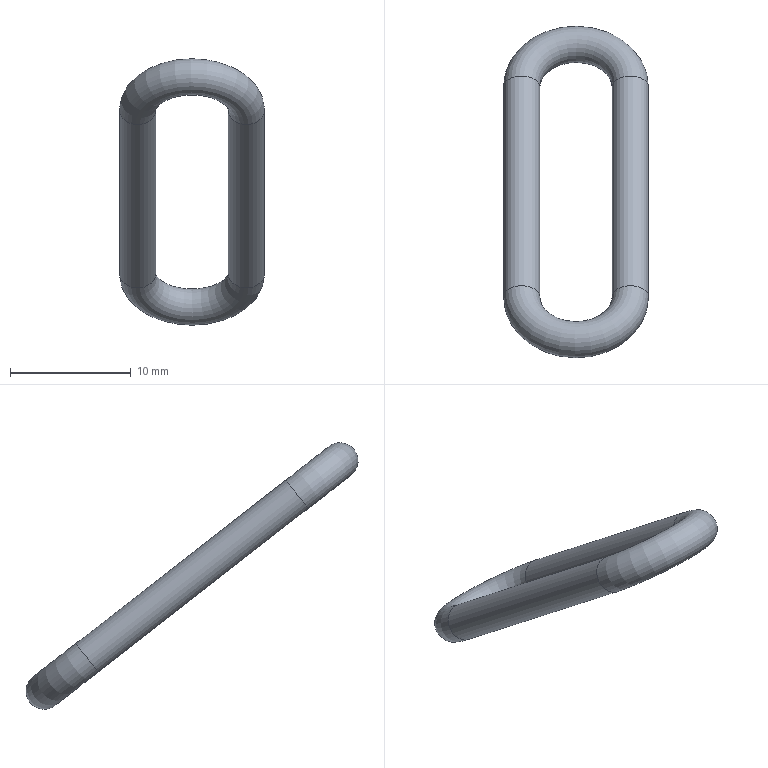Part | NX | features ACO1606-1-04.1 2 | 1 solid | 4 faces | box 12 x 27.465 x 22.038 mm | volume 510.877 mm3 | torus 2 | cylinder 2 | commonest cylinder face diameters 3 x2
STEP:
#1=CARTESIAN_POINT('',(858.667,-769.942,-191.489));
#2=VERTEX_POINT('',#1);
#3=CARTESIAN_POINT('',(860.167,-769.942,-191.489));
#4=DIRECTION('',(0.,-0.7892,0.6141));
#5=DIRECTION('',(-1.,0.,0.));
#6=AXIS2_PLACEMENT_3D('',#3,#4,#5);
#7=CIRCLE('',#6,1.5);
#8=EDGE_CURVE('',#2,#2,#7,.T.);
#9=ORIENTED_EDGE('',*,*,#8,.T.);
#10=EDGE_LOOP('',(#9));
#11=FACE_BOUND('',#10,.T.);
#12=CARTESIAN_POINT('',(867.667,-769.942,-191.489));
#13=VERTEX_POINT('',#12);
#14=CARTESIAN_POINT('',(869.167,-769.942,-191.489));
#15=DIRECTION('',(0.,0.7892,-0.6141));
#16=DIRECTION('',(-1.,0.,0.));
#17=AXIS2_PLACEMENT_3D('',#14,#15,#16);
#18=CIRCLE('',#17,1.5);
#19=EDGE_CURVE('',#13,#13,#18,.T.);
#20=ORIENTED_EDGE('',*,*,#19,.F.);
#21=EDGE_LOOP('',(#20));
#22=FACE_BOUND('',#21,.T.);
#23=CARTESIAN_POINT('',(864.667,-769.942,-191.489));
#24=DIRECTION('',(0.,-0.6141,-0.7892));
#25=DIRECTION('',(0.,-0.7892,0.6141));
#26=AXIS2_PLACEMENT_3D('',#23,#24,#25);
#27=TOROIDAL_SURFACE('',#26,4.5,1.5);
#28=ADVANCED_FACE('',(#11,#22),#27,.T.);
#29=ORIENTED_EDGE('',*,*,#8,.F.);
#30=EDGE_LOOP('',(#29));
#31=FACE_BOUND('',#30,.T.);
#32=CARTESIAN_POINT('',(858.667,-752.579,-205.));
#33=VERTEX_POINT('',#32);
#34=CARTESIAN_POINT('',(860.167,-752.579,-205.));
#35=DIRECTION('',(0.,-0.7892,0.6141));
#36=DIRECTION('',(-1.,0.,0.));
#37=AXIS2_PLACEMENT_3D('',#34,#35,#36);
#38=CIRCLE('',#37,1.5);
#39=EDGE_CURVE('',#33,#33,#38,.T.);
#40=ORIENTED_EDGE('',*,*,#39,.T.);
#41=EDGE_LOOP('',(#40));
#42=FACE_BOUND('',#41,.T.);
#43=CARTESIAN_POINT('',(860.167,-761.26,-198.245));
#44=DIRECTION('',(0.,-0.7892,0.6141));
#45=DIRECTION('',(0.,0.6141,0.7892));
#46=AXIS2_PLACEMENT_3D('',#43,#44,#45);
#47=CYLINDRICAL_SURFACE('',#46,1.5);
#48=ADVANCED_FACE('',(#31,#42),#47,.T.);
#49=CARTESIAN_POINT('',(867.667,-752.579,-205.));
#50=VERTEX_POINT('',#49);
#51=CARTESIAN_POINT('',(869.167,-752.579,-205.));
#52=DIRECTION('',(0.,0.7892,-0.6141));
#53=DIRECTION('',(-1.,0.,0.));
#54=AXIS2_PLACEMENT_3D('',#51,#52,#53);
#55=CIRCLE('',#54,1.5);
#56=EDGE_CURVE('',#50,#50,#55,.T.);
#57=ORIENTED_EDGE('',*,*,#56,.T.);
#58=EDGE_LOOP('',(#57));
#59=FACE_BOUND('',#58,.T.);
#60=ORIENTED_EDGE('',*,*,#39,.F.);
#61=EDGE_LOOP('',(#60));
#62=FACE_BOUND('',#61,.T.);
#63=CARTESIAN_POINT('',(864.667,-752.579,-205.));
#64=DIRECTION('',(0.,-0.6141,-0.7892));
#65=DIRECTION('',(0.,-0.7892,0.6141));
#66=AXIS2_PLACEMENT_3D('',#63,#64,#65);
#67=TOROIDAL_SURFACE('',#66,4.5,1.5);
#68=ADVANCED_FACE('',(#59,#62),#67,.T.);
#69=ORIENTED_EDGE('',*,*,#56,.F.);
#70=EDGE_LOOP('',(#69));
#71=FACE_BOUND('',#70,.T.);
#72=ORIENTED_EDGE('',*,*,#19,.T.);
#73=EDGE_LOOP('',(#72));
#74=FACE_BOUND('',#73,.T.);
#75=CARTESIAN_POINT('',(869.167,-761.26,-198.245));
#76=DIRECTION('',(0.,0.7892,-0.6141));
#77=DIRECTION('',(0.,-0.6141,-0.7892));
#78=AXIS2_PLACEMENT_3D('',#75,#76,#77);
#79=CYLINDRICAL_SURFACE('',#78,1.5);
#80=ADVANCED_FACE('',(#71,#74),#79,.T.);
#81=CLOSED_SHELL('',(#28,#48,#68,#80));
#82=MANIFOLD_SOLID_BREP('',#81);
#83=(LENGTH_UNIT()NAMED_UNIT(*)SI_UNIT(.MILLI.,.METRE.));
#84=UNCERTAINTY_MEASURE_WITH_UNIT(LENGTH_MEASURE(0.00001),#83,'','');
#85=(NAMED_UNIT(*)PLANE_ANGLE_UNIT()SI_UNIT($,.RADIAN.));
#86=(NAMED_UNIT(*)SI_UNIT($,.STERADIAN.)SOLID_ANGLE_UNIT());
#87=(GEOMETRIC_REPRESENTATION_CONTEXT(3)GLOBAL_UNCERTAINTY_ASSIGNED_CONTEXT((#84))GLOBAL_UNIT_ASSIGNED_CONTEXT((#83,#85,#86))REPRESENTATION_CONTEXT('',''));
#88=ADVANCED_BREP_SHAPE_REPRESENTATION('',(#82),#87);